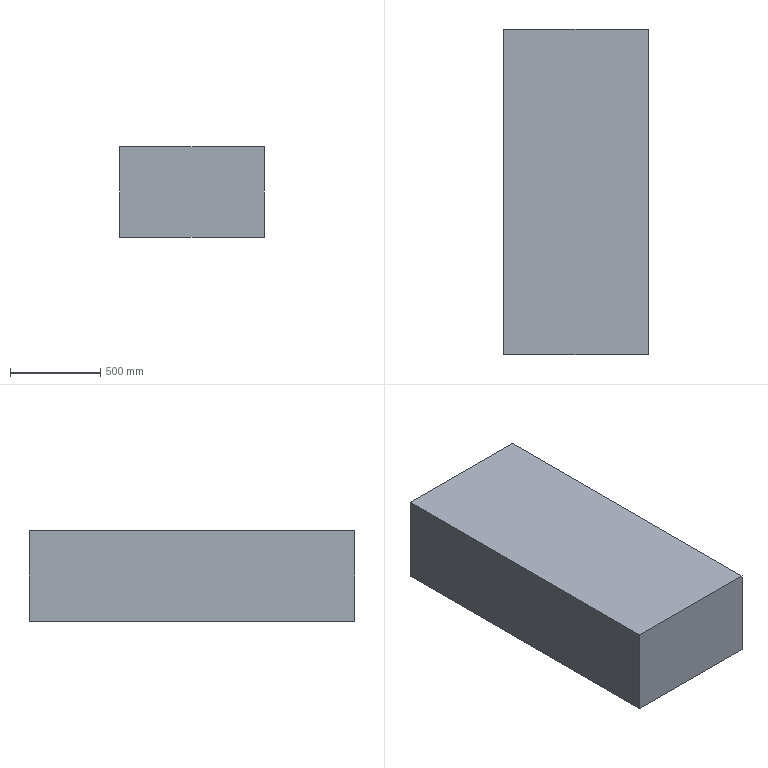Part | STEP file | Tool cabinet | 1 solid | 188 faces | box 800 x 1800 x 500 mm | volume 719981469 mm3 | plane 109 | spline 79